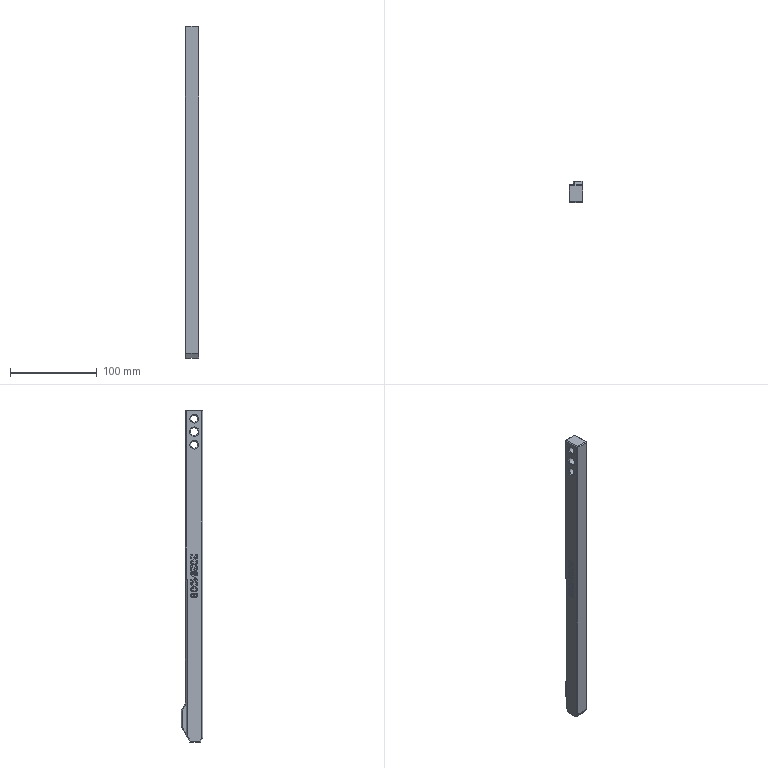Part | NX | features BREP 8, CHAMFER 2, solid 2, SUBTRACT 1 | 1 solid | 105 faces | box 16 x 25 x 382.34 mm | volume 118829 mm3 | plane 51 | spline 44 | cone 7 | cylinder 3 | commonest cylinder face diameters 8 x2 9 x1